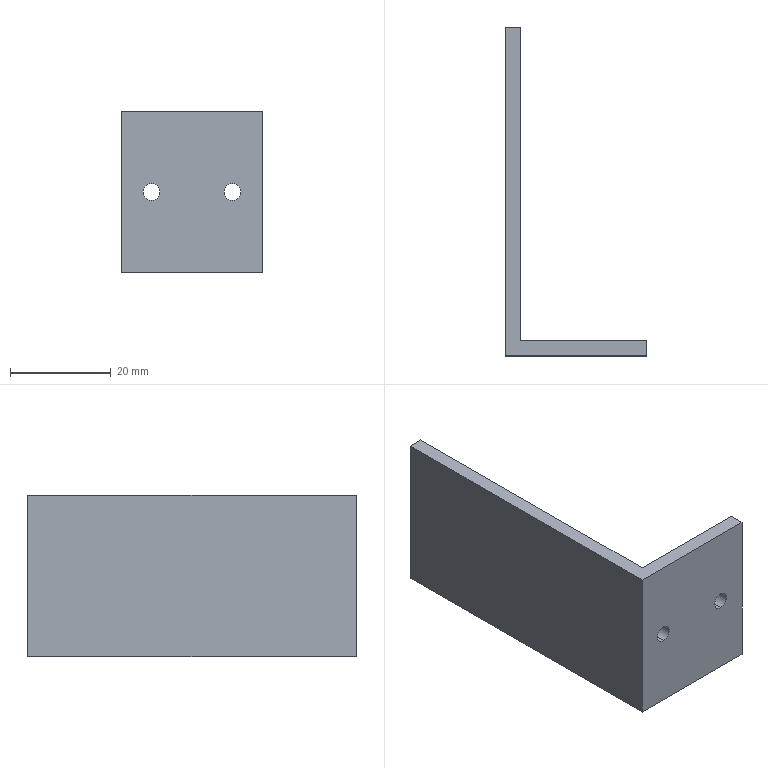Part | SolidWorks | features Extrusion 1, ICE 1 | 1 solid | 12 faces | box 28 x 65 x 32 mm | volume 8589 mm3 | plane 8 | cylinder 4 | commonest cylinder face diameters 3.3 x4
STEP:
#1=CARTESIAN_POINT('',(6.,0.,1.65));
#2=VERTEX_POINT('',#1);
#3=CARTESIAN_POINT('',(6.,0.,-1.65));
#4=VERTEX_POINT('',#3);
#5=CARTESIAN_POINT('',(6.,0.,0.));
#6=DIRECTION('',(0.,-1.,0.));
#7=DIRECTION('',(0.,0.,-1.));
#8=AXIS2_PLACEMENT_3D('',#5,#6,#7);
#9=CIRCLE('',#8,1.65);
#10=EDGE_CURVE('',#2,#4,#9,.T.);
#11=ORIENTED_EDGE('',*,*,#10,.T.);
#12=CARTESIAN_POINT('',(6.,3.,-1.65));
#13=VERTEX_POINT('',#12);
#14=CARTESIAN_POINT('',(6.,-7.5,-1.65));
#15=DIRECTION('',(0.,1.,0.));
#16=VECTOR('',#15,1000.);
#17=LINE('',#14,#16);
#18=EDGE_CURVE('',#4,#13,#17,.T.);
#19=ORIENTED_EDGE('',*,*,#18,.T.);
#20=CARTESIAN_POINT('',(6.,3.,1.65));
#21=VERTEX_POINT('',#20);
#22=CARTESIAN_POINT('',(6.,3.,0.));
#23=DIRECTION('',(0.,1.,0.));
#24=DIRECTION('',(0.,0.,1.));
#25=AXIS2_PLACEMENT_3D('',#22,#23,#24);
#26=CIRCLE('',#25,1.65);
#27=EDGE_CURVE('',#13,#21,#26,.T.);
#28=ORIENTED_EDGE('',*,*,#27,.T.);
#29=CARTESIAN_POINT('',(6.,-7.5,1.65));
#30=DIRECTION('',(0.,1.,0.));
#31=VECTOR('',#30,1000.);
#32=LINE('',#29,#31);
#33=EDGE_CURVE('',#2,#21,#32,.T.);
#34=ORIENTED_EDGE('',*,*,#33,.F.);
#35=EDGE_LOOP('',(#11,#19,#28,#34));
#36=FACE_OUTER_BOUND('',#35,.T.);
#37=CARTESIAN_POINT('',(6.,-7.5,0.));
#38=DIRECTION('',(0.,1.,0.));
#39=DIRECTION('',(0.,0.,1.));
#40=AXIS2_PLACEMENT_3D('',#37,#38,#39);
#41=CYLINDRICAL_SURFACE('',#40,1.65);
#42=ADVANCED_FACE('',(#36),#41,.F.);
#43=CARTESIAN_POINT('',(22.,0.,1.65));
#44=VERTEX_POINT('',#43);
#45=CARTESIAN_POINT('',(22.,0.,-1.65));
#46=VERTEX_POINT('',#45);
#47=CARTESIAN_POINT('',(22.,0.,0.));
#48=DIRECTION('',(0.,-1.,0.));
#49=DIRECTION('',(0.,0.,-1.));
#50=AXIS2_PLACEMENT_3D('',#47,#48,#49);
#51=CIRCLE('',#50,1.65);
#52=EDGE_CURVE('',#44,#46,#51,.T.);
#53=ORIENTED_EDGE('',*,*,#52,.T.);
#54=CARTESIAN_POINT('',(22.,3.,-1.65));
#55=VERTEX_POINT('',#54);
#56=CARTESIAN_POINT('',(22.,-7.5,-1.65));
#57=DIRECTION('',(0.,1.,0.));
#58=VECTOR('',#57,1000.);
#59=LINE('',#56,#58);
#60=EDGE_CURVE('',#46,#55,#59,.T.);
#61=ORIENTED_EDGE('',*,*,#60,.T.);
#62=CARTESIAN_POINT('',(22.,3.,1.65));
#63=VERTEX_POINT('',#62);
#64=CARTESIAN_POINT('',(22.,3.,0.));
#65=DIRECTION('',(0.,1.,0.));
#66=DIRECTION('',(0.,0.,1.));
#67=AXIS2_PLACEMENT_3D('',#64,#65,#66);
#68=CIRCLE('',#67,1.65);
#69=EDGE_CURVE('',#55,#63,#68,.T.);
#70=ORIENTED_EDGE('',*,*,#69,.T.);
#71=CARTESIAN_POINT('',(22.,-7.5,1.65));
#72=DIRECTION('',(0.,1.,0.));
#73=VECTOR('',#72,1000.);
#74=LINE('',#71,#73);
#75=EDGE_CURVE('',#44,#63,#74,.T.);
#76=ORIENTED_EDGE('',*,*,#75,.F.);
#77=EDGE_LOOP('',(#53,#61,#70,#76));
#78=FACE_OUTER_BOUND('',#77,.T.);
#79=CARTESIAN_POINT('',(22.,-7.5,0.));
#80=DIRECTION('',(0.,1.,0.));
#81=DIRECTION('',(0.,0.,1.));
#82=AXIS2_PLACEMENT_3D('',#79,#80,#81);
#83=CYLINDRICAL_SURFACE('',#82,1.65);
#84=ADVANCED_FACE('',(#78),#83,.F.);
#85=CARTESIAN_POINT('',(0.,65.,16.));
#86=VERTEX_POINT('',#85);
#87=CARTESIAN_POINT('',(0.,0.,16.));
#88=VERTEX_POINT('',#87);
#89=CARTESIAN_POINT('',(0.,65.,16.));
#90=DIRECTION('',(0.,-1.,0.));
#91=VECTOR('',#90,1000.);
#92=LINE('',#89,#91);
#93=EDGE_CURVE('',#86,#88,#92,.T.);
#94=ORIENTED_EDGE('',*,*,#93,.F.);
#95=CARTESIAN_POINT('',(0.,65.,-16.));
#96=VERTEX_POINT('',#95);
#97=CARTESIAN_POINT('',(0.,65.,-16.));
#98=DIRECTION('',(0.,0.,1.));
#99=VECTOR('',#98,1000.);
#100=LINE('',#97,#99);
#101=EDGE_CURVE('',#96,#86,#100,.T.);
#102=ORIENTED_EDGE('',*,*,#101,.F.);
#103=CARTESIAN_POINT('',(0.,0.,-16.));
#104=VERTEX_POINT('',#103);
#105=CARTESIAN_POINT('',(0.,65.,-16.));
#106=DIRECTION('',(0.,-1.,0.));
#107=VECTOR('',#106,1000.);
#108=LINE('',#105,#107);
#109=EDGE_CURVE('',#96,#104,#108,.T.);
#110=ORIENTED_EDGE('',*,*,#109,.T.);
#111=CARTESIAN_POINT('',(0.,0.,-16.));
#112=DIRECTION('',(0.,0.,1.));
#113=VECTOR('',#112,1000.);
#114=LINE('',#111,#113);
#115=EDGE_CURVE('',#104,#88,#114,.T.);
#116=ORIENTED_EDGE('',*,*,#115,.T.);
#117=EDGE_LOOP('',(#94,#102,#110,#116));
#118=FACE_OUTER_BOUND('',#117,.T.);
#119=CARTESIAN_POINT('',(0.,65.,-16.));
#120=DIRECTION('',(-1.,0.,0.));
#121=DIRECTION('',(0.,0.,1.));
#122=AXIS2_PLACEMENT_3D('',#119,#120,#121);
#123=PLANE('',#122);
#124=ADVANCED_FACE('',(#118),#123,.T.);
#125=CARTESIAN_POINT('',(3.,65.,16.));
#126=VERTEX_POINT('',#125);
#127=CARTESIAN_POINT('',(3.,65.,16.));
#128=DIRECTION('',(-1.,0.,0.));
#129=VECTOR('',#128,1000.);
#130=LINE('',#127,#129);
#131=EDGE_CURVE('',#126,#86,#130,.T.);
#132=ORIENTED_EDGE('',*,*,#131,.F.);
#133=CARTESIAN_POINT('',(3.,65.,-16.));
#134=VERTEX_POINT('',#133);
#135=CARTESIAN_POINT('',(3.,65.,-16.));
#136=DIRECTION('',(0.,0.,1.));
#137=VECTOR('',#136,1000.);
#138=LINE('',#135,#137);
#139=EDGE_CURVE('',#134,#126,#138,.T.);
#140=ORIENTED_EDGE('',*,*,#139,.F.);
#141=CARTESIAN_POINT('',(3.,65.,-16.));
#142=DIRECTION('',(-1.,0.,0.));
#143=VECTOR('',#142,1000.);
#144=LINE('',#141,#143);
#145=EDGE_CURVE('',#134,#96,#144,.T.);
#146=ORIENTED_EDGE('',*,*,#145,.T.);
#147=ORIENTED_EDGE('',*,*,#101,.T.);
#148=EDGE_LOOP('',(#132,#140,#146,#147));
#149=FACE_OUTER_BOUND('',#148,.T.);
#150=CARTESIAN_POINT('',(3.,65.,-16.));
#151=DIRECTION('',(0.,1.,0.));
#152=DIRECTION('',(0.,0.,1.));
#153=AXIS2_PLACEMENT_3D('',#150,#151,#152);
#154=PLANE('',#153);
#155=ADVANCED_FACE('',(#149),#154,.T.);
#156=CARTESIAN_POINT('',(3.,3.,16.));
#157=VERTEX_POINT('',#156);
#158=CARTESIAN_POINT('',(3.,3.,16.));
#159=DIRECTION('',(0.,1.,0.));
#160=VECTOR('',#159,1000.);
#161=LINE('',#158,#160);
#162=EDGE_CURVE('',#157,#126,#161,.T.);
#163=ORIENTED_EDGE('',*,*,#162,.F.);
#164=CARTESIAN_POINT('',(3.,3.,-16.));
#165=VERTEX_POINT('',#164);
#166=CARTESIAN_POINT('',(3.,3.,-16.));
#167=DIRECTION('',(0.,0.,1.));
#168=VECTOR('',#167,1000.);
#169=LINE('',#166,#168);
#170=EDGE_CURVE('',#165,#157,#169,.T.);
#171=ORIENTED_EDGE('',*,*,#170,.F.);
#172=CARTESIAN_POINT('',(3.,3.,-16.));
#173=DIRECTION('',(0.,1.,0.));
#174=VECTOR('',#173,1000.);
#175=LINE('',#172,#174);
#176=EDGE_CURVE('',#165,#134,#175,.T.);
#177=ORIENTED_EDGE('',*,*,#176,.T.);
#178=ORIENTED_EDGE('',*,*,#139,.T.);
#179=EDGE_LOOP('',(#163,#171,#177,#178));
#180=FACE_OUTER_BOUND('',#179,.T.);
#181=CARTESIAN_POINT('',(3.,3.,-16.));
#182=DIRECTION('',(1.,0.,0.));
#183=DIRECTION('',(0.,0.,-1.));
#184=AXIS2_PLACEMENT_3D('',#181,#182,#183);
#185=PLANE('',#184);
#186=ADVANCED_FACE('',(#180),#185,.T.);
#187=CARTESIAN_POINT('',(6.,3.,0.));
#188=DIRECTION('',(0.,1.,0.));
#189=DIRECTION('',(0.,0.,1.));
#190=AXIS2_PLACEMENT_3D('',#187,#188,#189);
#191=CIRCLE('',#190,1.65);
#192=EDGE_CURVE('',#21,#13,#191,.T.);
#193=ORIENTED_EDGE('',*,*,#192,.F.);
#194=ORIENTED_EDGE('',*,*,#27,.F.);
#195=EDGE_LOOP('',(#193,#194));
#196=FACE_BOUND('',#195,.T.);
#197=CARTESIAN_POINT('',(22.,3.,0.));
#198=DIRECTION('',(0.,1.,0.));
#199=DIRECTION('',(0.,0.,1.));
#200=AXIS2_PLACEMENT_3D('',#197,#198,#199);
#201=CIRCLE('',#200,1.65);
#202=EDGE_CURVE('',#63,#55,#201,.T.);
#203=ORIENTED_EDGE('',*,*,#202,.F.);
#204=ORIENTED_EDGE('',*,*,#69,.F.);
#205=EDGE_LOOP('',(#203,#204));
#206=FACE_BOUND('',#205,.T.);
#207=CARTESIAN_POINT('',(28.,3.,16.));
#208=VERTEX_POINT('',#207);
#209=CARTESIAN_POINT('',(28.,3.,16.));
#210=DIRECTION('',(-1.,0.,0.));
#211=VECTOR('',#210,1000.);
#212=LINE('',#209,#211);
#213=EDGE_CURVE('',#208,#157,#212,.T.);
#214=ORIENTED_EDGE('',*,*,#213,.F.);
#215=CARTESIAN_POINT('',(28.,3.,-16.));
#216=VERTEX_POINT('',#215);
#217=CARTESIAN_POINT('',(28.,3.,-16.));
#218=DIRECTION('',(0.,0.,1.));
#219=VECTOR('',#218,1000.);
#220=LINE('',#217,#219);
#221=EDGE_CURVE('',#216,#208,#220,.T.);
#222=ORIENTED_EDGE('',*,*,#221,.F.);
#223=CARTESIAN_POINT('',(28.,3.,-16.));
#224=DIRECTION('',(-1.,0.,0.));
#225=VECTOR('',#224,1000.);
#226=LINE('',#223,#225);
#227=EDGE_CURVE('',#216,#165,#226,.T.);
#228=ORIENTED_EDGE('',*,*,#227,.T.);
#229=ORIENTED_EDGE('',*,*,#170,.T.);
#230=EDGE_LOOP('',(#214,#222,#228,#229));
#231=FACE_OUTER_BOUND('',#230,.T.);
#232=CARTESIAN_POINT('',(28.,3.,-16.));
#233=DIRECTION('',(0.,1.,0.));
#234=DIRECTION('',(0.,0.,1.));
#235=AXIS2_PLACEMENT_3D('',#232,#233,#234);
#236=PLANE('',#235);
#237=ADVANCED_FACE('',(#196,#206,#231),#236,.T.);
#238=CARTESIAN_POINT('',(28.,0.,16.));
#239=VERTEX_POINT('',#238);
#240=CARTESIAN_POINT('',(28.,0.,16.));
#241=DIRECTION('',(0.,1.,0.));
#242=VECTOR('',#241,1000.);
#243=LINE('',#240,#242);
#244=EDGE_CURVE('',#239,#208,#243,.T.);
#245=ORIENTED_EDGE('',*,*,#244,.F.);
#246=CARTESIAN_POINT('',(28.,0.,-16.));
#247=VERTEX_POINT('',#246);
#248=CARTESIAN_POINT('',(28.,0.,-16.));
#249=DIRECTION('',(0.,0.,1.));
#250=VECTOR('',#249,1000.);
#251=LINE('',#248,#250);
#252=EDGE_CURVE('',#247,#239,#251,.T.);
#253=ORIENTED_EDGE('',*,*,#252,.F.);
#254=CARTESIAN_POINT('',(28.,0.,-16.));
#255=DIRECTION('',(0.,1.,0.));
#256=VECTOR('',#255,1000.);
#257=LINE('',#254,#256);
#258=EDGE_CURVE('',#247,#216,#257,.T.);
#259=ORIENTED_EDGE('',*,*,#258,.T.);
#260=ORIENTED_EDGE('',*,*,#221,.T.);
#261=EDGE_LOOP('',(#245,#253,#259,#260));
#262=FACE_OUTER_BOUND('',#261,.T.);
#263=CARTESIAN_POINT('',(28.,0.,-16.));
#264=DIRECTION('',(1.,0.,0.));
#265=DIRECTION('',(0.,0.,-1.));
#266=AXIS2_PLACEMENT_3D('',#263,#264,#265);
#267=PLANE('',#266);
#268=ADVANCED_FACE('',(#262),#267,.T.);
#269=ORIENTED_EDGE('',*,*,#10,.F.);
#270=CARTESIAN_POINT('',(6.,0.,0.));
#271=DIRECTION('',(0.,-1.,0.));
#272=DIRECTION('',(0.,0.,-1.));
#273=AXIS2_PLACEMENT_3D('',#270,#271,#272);
#274=CIRCLE('',#273,1.65);
#275=EDGE_CURVE('',#4,#2,#274,.T.);
#276=ORIENTED_EDGE('',*,*,#275,.F.);
#277=EDGE_LOOP('',(#269,#276));
#278=FACE_BOUND('',#277,.T.);
#279=ORIENTED_EDGE('',*,*,#52,.F.);
#280=CARTESIAN_POINT('',(22.,0.,0.));
#281=DIRECTION('',(0.,-1.,0.));
#282=DIRECTION('',(0.,0.,-1.));
#283=AXIS2_PLACEMENT_3D('',#280,#281,#282);
#284=CIRCLE('',#283,1.65);
#285=EDGE_CURVE('',#46,#44,#284,.T.);
#286=ORIENTED_EDGE('',*,*,#285,.F.);
#287=EDGE_LOOP('',(#279,#286));
#288=FACE_BOUND('',#287,.T.);
#289=CARTESIAN_POINT('',(0.,0.,16.));
#290=DIRECTION('',(1.,0.,0.));
#291=VECTOR('',#290,1000.);
#292=LINE('',#289,#291);
#293=EDGE_CURVE('',#88,#239,#292,.T.);
#294=ORIENTED_EDGE('',*,*,#293,.F.);
#295=ORIENTED_EDGE('',*,*,#115,.F.);
#296=CARTESIAN_POINT('',(0.,0.,-16.));
#297=DIRECTION('',(1.,0.,0.));
#298=VECTOR('',#297,1000.);
#299=LINE('',#296,#298);
#300=EDGE_CURVE('',#104,#247,#299,.T.);
#301=ORIENTED_EDGE('',*,*,#300,.T.);
#302=ORIENTED_EDGE('',*,*,#252,.T.);
#303=EDGE_LOOP('',(#294,#295,#301,#302));
#304=FACE_OUTER_BOUND('',#303,.T.);
#305=CARTESIAN_POINT('',(0.,0.,-16.));
#306=DIRECTION('',(0.,-1.,0.));
#307=DIRECTION('',(0.,0.,-1.));
#308=AXIS2_PLACEMENT_3D('',#305,#306,#307);
#309=PLANE('',#308);
#310=ADVANCED_FACE('',(#278,#288,#304),#309,.T.);
#311=ORIENTED_EDGE('',*,*,#109,.F.);
#312=ORIENTED_EDGE('',*,*,#145,.F.);
#313=ORIENTED_EDGE('',*,*,#176,.F.);
#314=ORIENTED_EDGE('',*,*,#227,.F.);
#315=ORIENTED_EDGE('',*,*,#258,.F.);
#316=ORIENTED_EDGE('',*,*,#300,.F.);
#317=EDGE_LOOP('',(#311,#312,#313,#314,#315,#316));
#318=FACE_OUTER_BOUND('',#317,.T.);
#319=CARTESIAN_POINT('',(0.,0.,-16.));
#320=DIRECTION('',(0.,0.,1.));
#321=DIRECTION('',(1.,0.,0.));
#322=AXIS2_PLACEMENT_3D('',#319,#320,#321);
#323=PLANE('',#322);
#324=ADVANCED_FACE('',(#318),#323,.F.);
#325=ORIENTED_EDGE('',*,*,#93,.T.);
#326=ORIENTED_EDGE('',*,*,#293,.T.);
#327=ORIENTED_EDGE('',*,*,#244,.T.);
#328=ORIENTED_EDGE('',*,*,#213,.T.);
#329=ORIENTED_EDGE('',*,*,#162,.T.);
#330=ORIENTED_EDGE('',*,*,#131,.T.);
#331=EDGE_LOOP('',(#325,#326,#327,#328,#329,#330));
#332=FACE_OUTER_BOUND('',#331,.T.);
#333=CARTESIAN_POINT('',(0.,0.,16.));
#334=DIRECTION('',(0.,0.,1.));
#335=DIRECTION('',(1.,0.,0.));
#336=AXIS2_PLACEMENT_3D('',#333,#334,#335);
#337=PLANE('',#336);
#338=ADVANCED_FACE('',(#332),#337,.T.);
#339=ORIENTED_EDGE('',*,*,#60,.F.);
#340=ORIENTED_EDGE('',*,*,#285,.T.);
#341=ORIENTED_EDGE('',*,*,#75,.T.);
#342=ORIENTED_EDGE('',*,*,#202,.T.);
#343=EDGE_LOOP('',(#339,#340,#341,#342));
#344=FACE_OUTER_BOUND('',#343,.T.);
#345=CARTESIAN_POINT('',(22.,-7.5,0.));
#346=DIRECTION('',(0.,1.,0.));
#347=DIRECTION('',(0.,0.,1.));
#348=AXIS2_PLACEMENT_3D('',#345,#346,#347);
#349=CYLINDRICAL_SURFACE('',#348,1.65);
#350=ADVANCED_FACE('',(#344),#349,.F.);
#351=ORIENTED_EDGE('',*,*,#18,.F.);
#352=ORIENTED_EDGE('',*,*,#275,.T.);
#353=ORIENTED_EDGE('',*,*,#33,.T.);
#354=ORIENTED_EDGE('',*,*,#192,.T.);
#355=EDGE_LOOP('',(#351,#352,#353,#354));
#356=FACE_OUTER_BOUND('',#355,.T.);
#357=CARTESIAN_POINT('',(6.,-7.5,0.));
#358=DIRECTION('',(0.,1.,0.));
#359=DIRECTION('',(0.,0.,1.));
#360=AXIS2_PLACEMENT_3D('',#357,#358,#359);
#361=CYLINDRICAL_SURFACE('',#360,1.65);
#362=ADVANCED_FACE('',(#356),#361,.F.);
#363=CLOSED_SHELL('',(#42,#84,#124,#155,#186,#237,#268,#310,#324,#338,#350,#362));
#364=MANIFOLD_SOLID_BREP('',#363);
#365=CARTESIAN_POINT('',(0.,0.,0.));
#366=DIRECTION('',(0.,0.,1.));
#367=DIRECTION('',(1.,0.,0.));
#368=AXIS2_PLACEMENT_3D('',#365,#366,#367);
#369=(LENGTH_UNIT()NAMED_UNIT(*)SI_UNIT(.MILLI.,.METRE.));
#370=UNCERTAINTY_MEASURE_WITH_UNIT(LENGTH_MEASURE(0.00001),#369,'','');
#371=(NAMED_UNIT(*)PLANE_ANGLE_UNIT()SI_UNIT($,.RADIAN.));
#372=(NAMED_UNIT(*)SI_UNIT($,.STERADIAN.)SOLID_ANGLE_UNIT());
#373=(GEOMETRIC_REPRESENTATION_CONTEXT(3)GLOBAL_UNCERTAINTY_ASSIGNED_CONTEXT((#370))GLOBAL_UNIT_ASSIGNED_CONTEXT((#369,#371,#372))REPRESENTATION_CONTEXT('',''));
#374=ADVANCED_BREP_SHAPE_REPRESENTATION('',(#364,#368),#373);